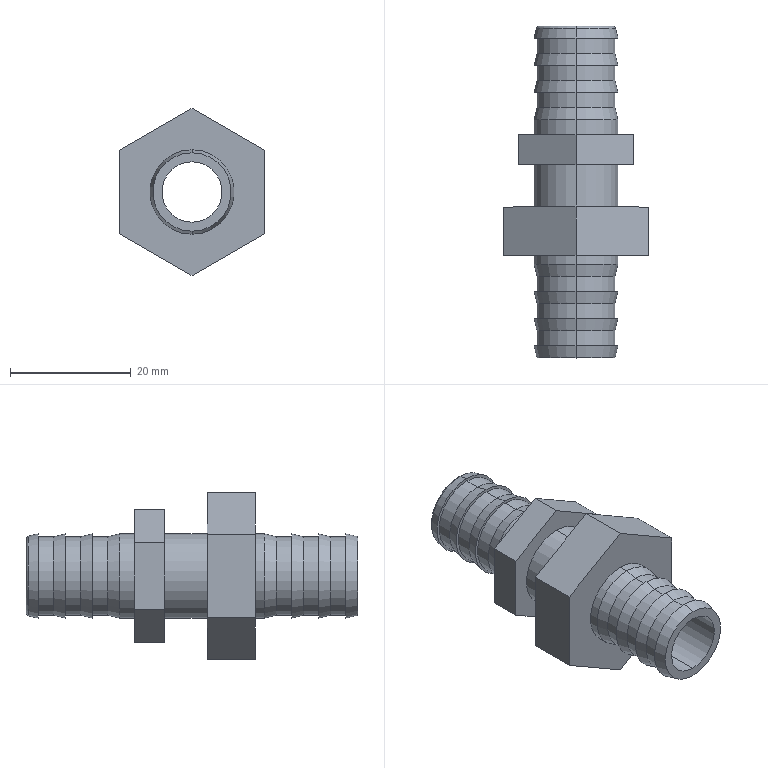Part | SolidWorks | features ICE 4, Extrusion 1, Fillet 1, RevCut 1 | 2 solids | 62 faces | box 24 x 55 x 27.713 mm | volume 7209 mm3 | plane 24 | cylinder 20 | cone 16 | torus 2 | commonest cylinder face diameters 13 x12 14 x6 10 x2